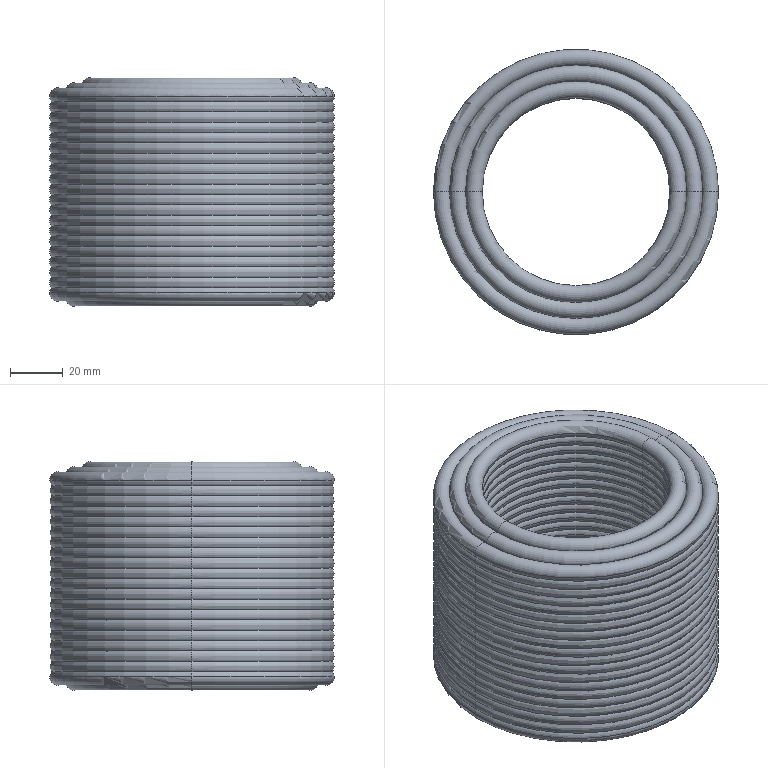Part | STEP file | Cable Rep^Pittsburgh Automotive 1300lb remote controlled electric hoist - Representation | 17 solids | 428 faces | box 107.694 x 107.694 x 86.428 mm | volume 372136 mm3 | torus 428